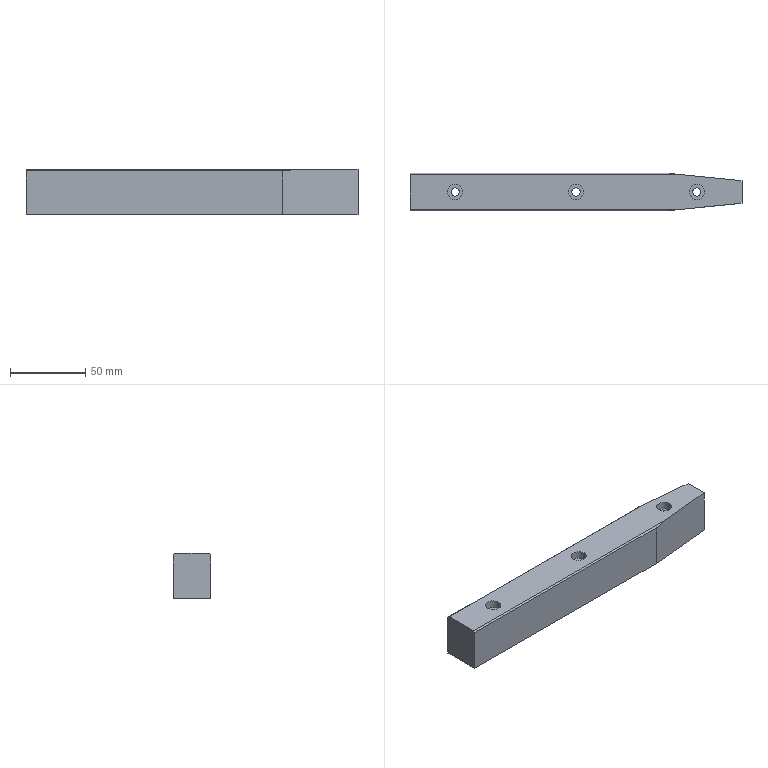Part | STEP file | 1 solid | 25 faces | box 220 x 25 x 30 mm | volume 154301 mm3 | plane 13 | cylinder 12 | commonest cylinder face diameters 5.5 x6 10 x6